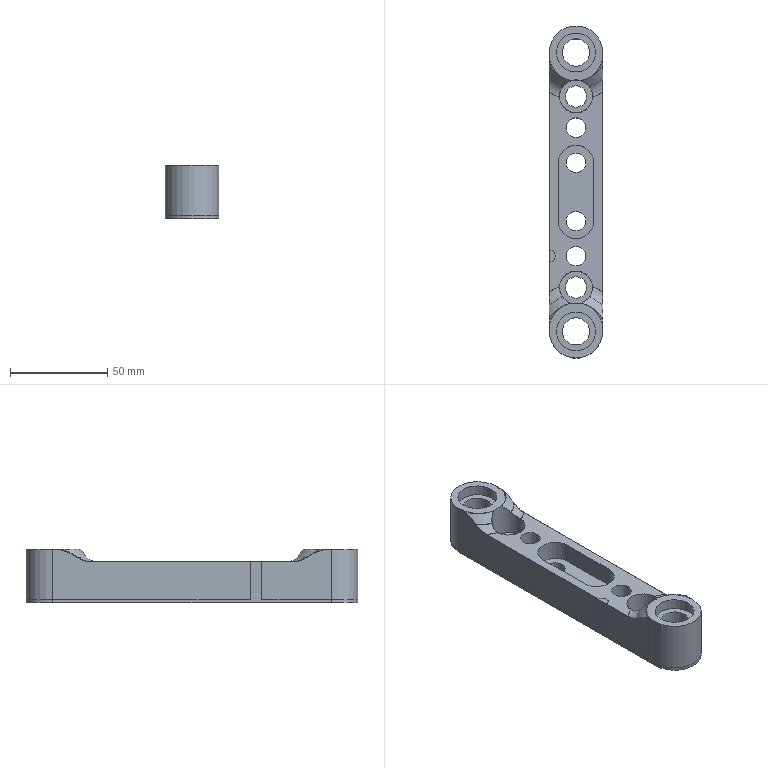NC program | NX | posted with a generic post | part box 27.4 x 170.48 x 27.5 mm
Lines 5462 to 6209 of 10888:
(ADAPTIVE_MILLING_COPY , TOOL : D8开粗)
N10886 T06 M6
N10888 G54
N10890 G17 G0 G90 X-73.84 Y2.769 B0. C0. S4000 M3
N10892 G43 Z30. H6
N10894 Z3.
N10896 G94 G3 X-73.84 Y2.769 Z2.605 I2.3 J-2.77 F1500.
N10898 X-73.84 Y2.769 Z2.21 I2.3 J-2.77
N10900 X-73.84 Y2.769 Z1.816 I2.3 J-2.77
N10902 X-73.84 Y2.769 Z1.421 I2.3 J-2.77
N10904 X-73.84 Y2.769 Z1.026 I2.3 J-2.77
N10906 X-73.84 Y2.769 Z0.631 I2.3 J-2.77
N10908 X-73.84 Y2.769 Z0.236 I2.3 J-2.77
N10910 X-73.84 Y2.769 Z-0.159 I2.3 J-2.77
N10912 X-73.84 Y2.769 Z-0.553 I2.3 J-2.77
N10914 X-73.84 Y2.769 Z-0.948 I2.3 J-2.77
N10916 X-73.84 Y2.769 Z-1.343 I2.3 J-2.77
N10918 X-73.84 Y2.769 Z-1.738 I2.3 J-2.77
N10920 X-73.84 Y2.769 Z-2.133 I2.3 J-2.77
N10922 X-73.84 Y2.769 Z-2.528 I2.3 J-2.77
N10924 X-73.84 Y2.769 Z-2.922 I2.3 J-2.77
N10926 X-73.84 Y2.769 Z-3.317 I2.3 J-2.77
N10928 X-73.84 Y2.769 Z-3.712 I2.3 J-2.77
N10930 X-73.84 Y2.769 Z-4.107 I2.3 J-2.77
N10932 X-73.84 Y2.769 Z-4.502 I2.3 J-2.77
N10934 X-71.541 Y3.599 Z-4.853 R-3.6
N10936 X-68.26 Y-1.603 R-3.625
N10938 X-74.92 Y-1.63 R-3.701
N10940 X-70.356 Y3.616 R-3.777
N10942 X-74.119 Y-2.909 R3.84
N10944 X-70.299 Y3.738 R-3.912
N10946 X-74.023 Y-3.163 R3.976
N10948 X-70.052 Y3.789 R-4.045
N10950 X-73.899 Y-3.423 R4.111
N10952 X-70.025 Y3.926 R-4.182
N10954 X-73.744 Y-3.685 R4.249
N10956 X-70.014 Y4.072 R-4.321
N10958 X-73.558 Y-3.949 R4.39
N10960 X-69.804 Y4.14 R-4.462
N10962 X-75.75 Y1.741 R4.533
N10964 X-73.34 Y-4.208 R4.533
N10966 X-69.824 Y4.306 R-4.606
N10968 X-72.864 Y-4.535 R-4.681
N10970 X-70.316 Y4.629 R-4.756
N10972 X-72.337 Y-4.809 R-4.832
N10974 X-71.101 Y4.925 R-4.909
N10976 X-71.272 Y-5.021 R-4.987
N10978 X-72.435 Y5.03 R-5.067
N10980 X-69.696 Y-4.845 R-5.148
N10982 X-74.43 Y4.417 R-5.229
N10984 X-67.181 Y-3.098 R-5.315
N10986 X-77.004 Y-0.069 R-5.404
N10988 X-66.868 Y2.951 R-5.495
N10990 X-75.057 Y-4.408 R-5.584
N10992 X-65.915 Y-0.707 R5.654
N10994 X-74.818 Y4.656 R5.678
N10996 X-76.45 Y2.889 R6.452
N10998 X-66.026 Y-1.422 R-5.695
N11000 X-65.913 Y0.863 R6.414
N11002 X-66.959 Y3.373 R6.034
N11004 X-69.395 Y5.276 R5.646
N11006 X-70.5 Y4.622 R0.808
N11008 G1 X-70.622 Y3.585
N11010 X-70.64 Y3.436 Z-4.849
N11012 X-70.657 Y3.287 Z-4.838
N11014 X-70.675 Y3.138 Z-4.819
N11016 X-70.693 Y2.989 Z-4.792
N11018 X-70.71 Y2.84 Z-4.758
N11020 X-70.728 Y2.691 Z-4.715
N11022 X-70.745 Y2.542 Z-4.663
N11024 X-70.763 Y2.393 Z-4.602
N11026 X-70.781 Y2.245 Z-4.532
N11028 X-70.798 Y2.096 Z-4.451
N11030 X-70.816 Y1.947 Z-4.358
N11032 X-70.833 Y1.798 Z-4.253
N11034 X-70.851 Y1.649 Z-4.133
N11036 X-70.869 Y1.5 Z-3.995
N11038 X-70.886 Y1.351 Z-3.837
N11040 X-70.904 Y1.202 Z-3.653
N11042 X-70.921 Y1.053 Z-3.433
N11044 X-70.939 Y0.904 Z-3.161
N11046 X-70.956 Y0.755 Z-2.79
N11048 X-70.974 Y0.606 Z-1.853
N11050 G0 Z30.
N11052 X69.239 Y2.771
N11054 Z3.
N11056 G3 X69.239 Y2.771 Z2.605 I2.3 J-2.77
N11058 X69.239 Y2.771 Z2.21 I2.3 J-2.77
N11060 X69.239 Y2.771 Z1.816 I2.3 J-2.77
N11062 X69.239 Y2.771 Z1.421 I2.3 J-2.77
N11064 X69.239 Y2.771 Z1.026 I2.3 J-2.77
N11066 X69.239 Y2.771 Z0.631 I2.3 J-2.77
N11068 X69.239 Y2.771 Z0.236 I2.3 J-2.77
N11070 X69.239 Y2.771 Z-0.159 I2.3 J-2.77
N11072 X69.239 Y2.771 Z-0.553 I2.3 J-2.77
N11074 X69.239 Y2.771 Z-0.948 I2.3 J-2.77
N11076 X69.239 Y2.771 Z-1.343 I2.3 J-2.77
N11078 X69.239 Y2.771 Z-1.738 I2.3 J-2.77
N11080 X69.239 Y2.771 Z-2.133 I2.3 J-2.77
N11082 X69.239 Y2.771 Z-2.528 I2.3 J-2.77
N11084 X69.239 Y2.771 Z-2.922 I2.3 J-2.77
N11086 X69.239 Y2.771 Z-3.317 I2.3 J-2.77
N11088 X69.239 Y2.771 Z-3.712 I2.3 J-2.77
N11090 X69.239 Y2.771 Z-4.107 I2.3 J-2.77
N11092 X69.239 Y2.771 Z-4.502 I2.3 J-2.77
N11094 X71.539 Y3.601 Z-4.853 R-3.6
N11096 X74.82 Y-1.601 R-3.625
N11098 X68.16 Y-1.627 R-3.701
N11100 X72.723 Y3.617 R-3.777
N11102 X68.803 Y-2.759 R3.839
N11104 X72.572 Y3.806 R-3.912
N11106 X69.234 Y-3.292 R3.977
N11108 X72.819 Y3.87 R-4.046
N11110 X69.182 Y-3.422 R4.112
N11112 X73.053 Y3.929 R-4.182
N11114 X69.146 Y-3.563 R4.249
N11116 X73.064 Y4.075 R-4.32
N11118 X69.123 Y-3.716 R4.389
N11120 X73.275 Y4.142 R-4.461
N11122 X69.525 Y-4.11 R4.533
N11124 X73.036 Y4.39 R-4.607
N11126 X69.764 Y-4.376 R4.68
N11128 X72.766 Y4.628 R-4.755
N11130 X66.845 Y1.221 R4.831
N11132 X70.267 Y-4.704 R4.831
N11134 X72.224 Y4.895 R-4.907
N11136 X71.312 Y-5.02 R-4.985
N11138 X71.388 Y5.1 R-5.063
N11140 X72.905 Y-4.998 R-5.144
N11142 X69.316 Y4.783 R-5.226
N11144 X75.409 Y-3.684 R-5.31
N11146 X66.354 Y1.7 R-5.398
N11148 X76.959 Y1.04 R-5.488
N11150 X67.106 Y-3.479 R-5.578
N11152 X77.164 Y-0.712 R5.653
N11154 X71.272 Y5.688 R5.681
N11156 X66.021 Y1.396 R5.729
N11158 X67.16 Y-3.638 R5.816
N11160 X74.269 Y-4.999 R5.748
N11162 X76.644 Y-2.519 R6.075
N11164 X77.231 Y-0.106 R6.229
N11166 X77.084 Y1.308 R7.829
N11168 X73.315 Y5.41 R5.784
N11170 X72.26 Y4.682 R0.808
N11172 G1 X72.207 Y3.631
N11174 X72.199 Y3.481 Z-4.849
N11176 X72.191 Y3.332 Z-4.838
N11178 X72.184 Y3.182 Z-4.819
N11180 X72.176 Y3.032 Z-4.792
N11182 X72.169 Y2.882 Z-4.758
N11184 X72.161 Y2.732 Z-4.715
N11186 X72.153 Y2.583 Z-4.663
N11188 X72.146 Y2.433 Z-4.602
N11190 X72.138 Y2.283 Z-4.532
N11192 X72.13 Y2.133 Z-4.451
N11194 X72.123 Y1.983 Z-4.358
N11196 X72.115 Y1.833 Z-4.253
N11198 X72.108 Y1.684 Z-4.133
N11200 X72.1 Y1.534 Z-3.995
N11202 X72.092 Y1.384 Z-3.837
N11204 X72.085 Y1.234 Z-3.653
N11206 X72.077 Y1.084 Z-3.433
N11208 X72.069 Y0.935 Z-3.161
N11210 X72.062 Y0.785 Z-2.79
N11212 X72.054 Y0.635 Z-1.853
N11214 G0 Z30.
N11216 X-46.689 Y-2.761
N11218 Z3.
N11220 G3 X-46.689 Y-2.761 Z2.605 I-2.311 J2.76
N11222 X-46.689 Y-2.761 Z2.21 I-2.311 J2.76
N11224 X-46.689 Y-2.761 Z1.816 I-2.311 J2.76
N11226 X-46.689 Y-2.761 Z1.421 I-2.311 J2.76
N11228 X-46.689 Y-2.761 Z1.026 I-2.311 J2.76
N11230 X-46.689 Y-2.761 Z0.631 I-2.311 J2.76
N11232 X-46.689 Y-2.761 Z0.236 I-2.311 J2.76
N11234 X-46.689 Y-2.761 Z-0.159 I-2.311 J2.76
N11236 X-46.689 Y-2.761 Z-0.553 I-2.311 J2.76
N11238 X-46.689 Y-2.761 Z-0.948 I-2.311 J2.76
N11240 X-46.689 Y-2.761 Z-1.343 I-2.311 J2.76
N11242 X-46.689 Y-2.761 Z-1.738 I-2.311 J2.76
N11244 X-46.689 Y-2.761 Z-2.133 I-2.311 J2.76
N11246 X-46.689 Y-2.761 Z-2.528 I-2.311 J2.76
N11248 X-46.689 Y-2.761 Z-2.922 I-2.311 J2.76
N11250 X-46.689 Y-2.761 Z-3.317 I-2.311 J2.76
N11252 X-46.689 Y-2.761 Z-3.712 I-2.311 J2.76
N11254 X-46.689 Y-2.761 Z-4.107 I-2.311 J2.76
N11256 X-46.689 Y-2.761 Z-4.502 I-2.311 J2.76
N11258 X-46.689 Y-2.761 Z-4.896 I-2.311 J2.76
N11260 X-46.689 Y-2.761 Z-5.291 I-2.311 J2.76
N11262 X-46.689 Y-2.761 Z-5.686 I-2.311 J2.76
N11264 X-46.689 Y-2.761 Z-6.081 I-2.311 J2.76
N11266 X-46.689 Y-2.761 Z-6.476 I-2.311 J2.76
N11268 X-46.689 Y-2.761 Z-6.871 I-2.311 J2.76
N11270 X-46.689 Y-2.761 Z-7.265 I-2.311 J2.76
N11272 X-46.689 Y-2.761 Z-7.66 I-2.311 J2.76
N11274 X-46.689 Y-2.761 Z-8.055 I-2.311 J2.76
N11276 X-46.689 Y-2.761 Z-8.45 I-2.311 J2.76
N11278 X-46.689 Y-2.761 Z-8.845 I-2.311 J2.76
N11280 X-46.689 Y-2.761 Z-9.24 I-2.311 J2.76
N11282 X-46.689 Y-2.761 Z-9.634 I-2.311 J2.76
N11284 X-46.689 Y-2.761 Z-10.029 I-2.311 J2.76
N11286 X-46.689 Y-2.761 Z-10.424 I-2.311 J2.76
N11288 X-46.689 Y-2.761 Z-10.819 I-2.311 J2.76
N11290 X-46.689 Y-2.761 Z-11.214 I-2.311 J2.76
N11292 X-46.689 Y-2.761 Z-11.608 I-2.311 J2.76
N11294 X-46.689 Y-2.761 Z-12.003 I-2.311 J2.76
N11296 X-46.689 Y-2.761 Z-12.398 I-2.311 J2.76
N11298 X-46.689 Y-2.761 Z-12.793 I-2.311 J2.76
N11300 X-46.689 Y-2.761 Z-13.188 I-2.311 J2.76
N11302 X-46.689 Y-2.761 Z-13.583 I-2.311 J2.76
N11304 X-46.689 Y-2.761 Z-13.977 I-2.311 J2.76
N11306 X-46.689 Y-2.761 Z-14.372 I-2.311 J2.76
N11308 X-46.689 Y-2.761 Z-14.767 I-2.311 J2.76
N11310 X-46.689 Y-2.761 Z-15.162 I-2.311 J2.76
N11312 X-46.689 Y-2.761 Z-15.557 I-2.311 J2.76
N11314 X-46.689 Y-2.761 Z-15.952 I-2.311 J2.76
N11316 X-46.689 Y-2.761 Z-16.346 I-2.311 J2.76
N11318 X-49. Y3.6 Z-16.5 R3.6
N11320 X-45.719 Y-1.602 R-3.625
N11322 X-52.283 Y-1.818 R-3.701
N11324 X-47.816 Y3.616 R-3.778
N11326 X-51.736 Y-2.76 R3.838
N11328 X-47.76 Y3.738 R-3.911
N11330 X-51.65 Y-3.021 R3.972
N11332 X-47.514 Y3.789 R-4.044
N11334 X-51.709 Y-3.149 R4.107
N11336 X-48.604 Y-4.149 R4.159
N11338 X-50.93 Y3.721 R-4.18
N11340 X-53.159 Y-0.53 R4.22
N11342 X-52.029 Y-2.882 R4.227
N11344 X-50.296 Y-3.988 R3.884
N11346 X-47.443 Y-3.89 R4.401
N11348 X-44.825 Y-0.368 R4.251
N11350 X-47.407 Y3.877 R4.225
N11352 X-48.508 Y3.221 R0.808
N11354 G1 X-48.634 Y2.16
N11356 X-48.652 Y2.011 Z-16.496
N11358 X-48.67 Y1.862 Z-16.485
N11360 X-48.687 Y1.713 Z-16.466
N11362 X-48.705 Y1.564 Z-16.439
N11364 X-48.723 Y1.415 Z-16.405
N11366 X-48.74 Y1.266 Z-16.362
N11368 X-48.758 Y1.117 Z-16.31
N11370 X-48.776 Y0.968 Z-16.25
N11372 X-48.794 Y0.819 Z-16.179
N11374 X-48.811 Y0.67 Z-16.098
N11376 X-48.829 Y0.521 Z-16.005
N11378 X-48.847 Y0.372 Z-15.9
N11380 X-48.864 Y0.223 Z-15.78
N11382 X-48.882 Y0.074 Z-15.642
N11384 X-48.9 Y-0.075 Z-15.484
N11386 X-48.917 Y-0.224 Z-15.3
N11388 X-48.935 Y-0.373 Z-15.08
N11390 X-48.953 Y-0.522 Z-14.808
N11392 X-48.97 Y-0.67 Z-14.437
N11394 X-48.988 Y-0.819 Z-13.5
N11396 G0 Z30.
N11398 X-48.921 Y0.758
N11400 Z-2.824
N11402 G1 X-48.949 Y0.611 Z-3.76
N11404 X-48.978 Y0.463 Z-4.131
N11406 X-49.006 Y0.316 Z-4.404
N11408 X-49.035 Y0.169 Z-4.624
N11410 X-49.063 Y0.021 Z-4.808
N11412 X-49.091 Y-0.126 Z-4.966
N11414 X-49.12 Y-0.273 Z-5.103
N11416 X-49.148 Y-0.421 Z-5.224
N11418 X-49.176 Y-0.568 Z-5.329
N11420 X-49.205 Y-0.715 Z-5.422
N11422 X-49.233 Y-0.862 Z-5.503
N11424 X-49.261 Y-1.01 Z-5.573
N11426 X-49.29 Y-1.157 Z-5.634
N11428 X-49.318 Y-1.304 Z-5.685
N11430 X-49.347 Y-1.452 Z-5.728
N11432 X-49.375 Y-1.599 Z-5.763
N11434 X-49.403 Y-1.746 Z-5.79
N11436 X-49.432 Y-1.893 Z-5.808
N11438 X-49.46 Y-2.041 Z-5.82
N11440 X-49.488 Y-2.188 Z-5.824
N11442 X-49.758 Y-3.586
N11444 G3 X-49.407 Y-4.414 R0.809
N11446 G2 X-47.983 Y-5.539 R6.465
N11448 X-47.123 Y-7.109 R4.659
N11450 X-47.037 Y-8.898 R4.659
N11452 X-48.987 Y-13.563 R17.207
N11454 X-50.821 Y-15.909 R7.143
N11456 X-51.757 Y-16.934 R6.606
N11458 G1 X-52.621 Y-17.475
N11460 G2 X-53.772 Y-17.834 R7.888
N11462 G3 X-54.224 Y-19.168 R0.8
N11464 X-53.705 Y-19.423 Z-5.786 R0.859
N11466 G1 X-52.722 Y-19.601 Z-5.724
N11468 X-51.383 Y-19.843 F15000.
N11470 G3 X-50.675 Y-19.622 R0.802
N11472 G1 X-49.772 Y-18.721
N11474 X-48.88 Y-17.81
N11476 G3 X-46.917 Y-15.066 R13.735
N11478 G1 X-45.249 Y-11.995
N11480 G3 X-45.158 Y-11.511 R0.81
N11482 G1 X-45.332 Y-10.155
N11484 X-45.488 Y-8.97 Z-5.799 F1500.
N11486 G3 X-45.654 Y-8.617 Z-5.824 R0.815
N11488 X-47.037 Y-8.898 R0.8
N11490 G1 X-47.296 Y-9.762
N11492 X-48.34 Y-12.034
N11494 X-49.59 Y-14.187
N11496 X-50.856 Y-15.955
N11498 G3 X-50.824 Y-16.938 R0.808
N11500 G1 X-49.981 Y-17.965
N11502 X-49.886 Y-18.081 Z-5.82
N11504 X-49.79 Y-18.197 Z-5.808
N11506 X-49.695 Y-18.313 Z-5.79
N11508 X-49.6 Y-18.429 Z-5.763
N11510 X-49.505 Y-18.545 Z-5.728
N11512 X-49.41 Y-18.661 Z-5.685
N11514 X-49.314 Y-18.777 Z-5.634
N11516 X-49.219 Y-18.892 Z-5.573
N11518 X-49.124 Y-19.008 Z-5.503
N11520 X-49.029 Y-19.124 Z-5.422
N11522 X-48.934 Y-19.24 Z-5.329
N11524 X-48.839 Y-19.356 Z-5.224
N11526 X-48.743 Y-19.472 Z-5.103
N11528 X-48.648 Y-19.588 Z-4.966
N11530 X-48.553 Y-19.704 Z-4.808
N11532 X-48.458 Y-19.82 Z-4.624
N11534 X-48.363 Y-19.936 Z-4.404
N11536 X-48.267 Y-20.052 Z-4.131
N11538 X-48.172 Y-20.168 Z-3.76
N11540 X-48.077 Y-20.284 Z-2.824
N11542 G0 Z30.
N11544 X-47.959 Y0.175
N11546 Z-1.853
N11548 G1 X-48.068 Y0.071 Z-2.79
N11550 X-48.176 Y-0.033 Z-3.161
N11552 X-48.284 Y-0.137 Z-3.433
N11554 X-48.392 Y-0.241 Z-3.653
N11556 X-48.501 Y-0.345 Z-3.837
N11558 X-48.609 Y-0.448 Z-3.995
N11560 X-48.717 Y-0.552 Z-4.133
N11562 X-48.825 Y-0.656 Z-4.253
N11564 X-48.934 Y-0.76 Z-4.358
N11566 X-49.042 Y-0.864 Z-4.451
N11568 X-49.15 Y-0.968 Z-4.532
N11570 X-49.258 Y-1.071 Z-4.602
N11572 X-49.367 Y-1.175 Z-4.663
N11574 X-49.475 Y-1.279 Z-4.715
N11576 X-49.583 Y-1.383 Z-4.758
N11578 X-49.691 Y-1.487 Z-4.792
N11580 X-49.799 Y-1.591 Z-4.819
N11582 X-49.908 Y-1.695 Z-4.838
N11584 X-50.016 Y-1.798 Z-4.849
N11586 X-50.124 Y-1.902 Z-4.853
N11588 X-50.877 Y-2.624
N11590 G3 X-50.788 Y-3.864 R0.808
N11592 G2 X-49.389 Y-4.957 R7.32
N11594 X-48.139 Y-8.974 R5.437
N11596 X-49.59 Y-13.357 R10.542
N11598 X-51.081 Y-15.5 R9.698
N11600 X-54.173 Y-17.113 R5.957
N11602 G1 X-54.468 Y-17.163
N11604 G3 X-54.874 Y-18.349 R0.8
N11606 X-54.229 Y-18.72 Z-4.804 R0.831
N11608 G1 X-53.419 Y-18.824 Z-4.753
N11610 X-51.831 Y-19.029 F15000.
N11612 G3 X-51.371 Y-18.951 R0.813
N11614 G1 X-51.039 Y-18.785
N11616 X-50.712 Y-18.609
N11618 G3 X-50.146 Y-18.141 R2.814
N11620 G1 X-49.146 Y-17.04
N11622 G3 X-47.722 Y-15.022 R13.499
N11624 G1 X-46.991 Y-13.731
N11626 G3 X-45.702 Y-9.541 R12.053
N11628 G1 X-45.636 Y-8.975
N11630 X-45.58 Y-8.407
N11632 G3 X-46.22 Y-5.513 R5.51
N11634 G1 X-47.029 Y-3.995
N11636 G3 X-47.42 Y-3.636 R0.807
N11638 G1 X-48.61 Y-3.128
N11640 X-49.247 Y-2.853 Z-4.797 F1500.
N11642 X-49.889 Y-2.588 Z-4.84
N11644 X-49.986 Y-2.563 Z-4.847
N11646 X-50.085 Y-2.547 Z-4.853
N11648 G3 X-50.605 Y-3.995 R0.8
N11650 G2 X-49.406 Y-5.36 R4.728
N11652 G1 X-49.281 Y-5.504
N11654 G2 X-48.811 Y-6.618 R5.434
N11656 X-49.444 Y-12.028 R9.131
N11658 X-51.782 Y-15.275 R7.349
N11660 X-52.871 Y-15.927 R4.
N11662 G1 X-53.231 Y-16.028
N11664 G3 X-53.433 Y-17.303 R0.8
N11666 X-52.692 Y-17.525 Z-4.802 R0.832
N11668 G1 X-51.914 Y-17.431 Z-4.753
N11670 X-50.841 Y-17.302 F15000.
N11672 G3 X-50.208 Y-16.838 R0.801
N11674 G1 X-46.169 Y-7.93
N11676 G3 X-46.292 Y-7.077 R0.801
N11678 G1 X-46.826 Y-6.458
N11680 X-47.192 Y-6.027 Z-4.789 F1500.
N11682 X-47.569 Y-5.607 Z-4.824
N11684 G3 X-47.982 Y-5.419 Z-4.853 R0.833
N11686 X-48.879 Y-6.365 R0.8
N11688 G1 X-48.696 Y-7.298
N11690 G2 X-49.35 Y-10.718 R9.889
N11692 X-51.161 Y-13.887 R7.958
N11694 X-51.926 Y-14.418 R1.888
N11696 G3 X-51.719 Y-15.869 R0.8
N11698 X-51.087 Y-15.785 Z-4.812 R0.847
N11700 G1 X-50.244 Y-15.379 Z-4.753
N11702 X-48.569 Y-14.573 F15000.
N11704 X-48.454 Y-14.504
N11706 X-48.35 Y-14.418
N11708 X-48.105 Y-14.174
N11710 X-47.868 Y-13.923
N11712 G3 X-47.508 Y-13.239 R1.968
N11714 G1 X-46.953 Y-11.344
N11716 X-46.927 Y-11.195
N11718 X-46.925 Y-11.043
N11720 X-47.064 Y-9.597
N11722 X-47.19 Y-8.336 Z-4.833 F1500.
N11724 X-47.233 Y-8.182 Z-4.843
N11726 X-47.306 Y-8.038 Z-4.853
N11728 G3 X-48.741 Y-8.247 R0.8
N11730 G1 X-49.014 Y-9.158
N11732 X-49.029 Y-9.192
N11734 X-49.059 Y-9.261
N11736 G3 X-47.42 Y-9.905 R-0.881
N11738 X-49.045 Y-9.226 R-0.88
N11740 X-48.04 Y-10.396 R0.83
N11742 X-47.605 Y-9.117 R0.875
N11744 X-49.075 Y-9.295 R0.83
N11746 G1 X-49.093 Y-9.428
N11748 X-49.092 Y-9.562
N11750 X-48.919 Y-11.196
N11752 X-48.805 Y-12.219 Z-4.788
N11754 G3 X-48.528 Y-12.692 Z-4.753 R0.802
N11756 X-47.272 Y-12.357 R0.801 F15000.
N11758 X-47.213 Y-11.933 R0.818
N11760 G1 X-47.411 Y-10.45
N11762 X-47.553 Y-9.427 Z-4.818 F1500.
N11764 G3 X-47.839 Y-8.964 Z-4.853 R0.802
N11766 X-49.06 Y-9.26 R0.8
N11768 G1 X-49.147 Y-9.546
N11770 G3 X-48.83 Y-8.989 R-0.797
N11772 X-49.076 Y-9.294 R0.831
N11774 X-49.374 Y-10.258 R3.935
N11776 G2 X-50.275 Y-12.355 R10.996
N11778 G3 X-50.319 Y-13.032 R0.802
N11780 X-49.325 Y-13.505 Z-4.777 R0.814
N11782 G1 X-48.955 Y-13.422 Z-4.753
N11784 X-47.319 Y-13.055 F15000.
N11786 G3 X-46.699 Y-12.355 R0.801
N11788 G1 X-46.674 Y-12.118
N11790 X-46.68 Y-11.879
N11792 X-46.708 Y-11.774
N11794 X-46.746 Y-11.672
N11796 X-47.367 Y-10.365
N11798 X-47.581 Y-9.907 Z-4.785 F1500.
N11800 X-47.808 Y-9.456 Z-4.817
N11802 G3 X-48.269 Y-9.127 Z-4.853 R0.821
N11804 X-49.201 Y-9.567 R0.8
N11806 G2 X-51.416 Y-13.638 R27.243
N11808 X-53.898 Y-16.683 R26.39
N11810 X-55.596 Y-17.679 R4.037
N11812 G3 X-56.556 Y-17.915 R8.77
N11814 X-57.269 Y-18.893 R0.808
N11816 G1 X-57.036 Y-19.956
N11818 X-57.003 Y-20.103 Z-4.849
N11820 X-56.971 Y-20.249 Z-4.838
N11822 X-56.939 Y-20.396 Z-4.819
N11824 X-56.907 Y-20.542 Z-4.792
N11826 X-56.875 Y-20.689 Z-4.758
N11828 X-56.843 Y-20.835 Z-4.715
N11830 X-56.81 Y-20.982 Z-4.663
N11832 X-56.778 Y-21.128 Z-4.602
N11834 X-56.746 Y-21.275 Z-4.532
N11836 X-56.714 Y-21.422 Z-4.451
N11838 X-56.682 Y-21.568 Z-4.358
N11840 X-56.65 Y-21.715 Z-4.253
N11842 X-56.617 Y-21.861 Z-4.133
N11844 X-56.585 Y-22.008 Z-3.995
N11846 X-56.553 Y-22.154 Z-3.837
N11848 X-56.521 Y-22.301 Z-3.653
N11850 X-56.489 Y-22.447 Z-3.433
N11852 X-56.456 Y-22.594 Z-3.161
N11854 X-56.424 Y-22.74 Z-2.79
N11856 X-56.392 Y-22.887 Z-1.853
N11858 G0 Z30.
N11860 X-54.862 Y22.912
N11862 Z-2.824
N11864 G1 X-54.844 Y22.763 Z-3.76
N11866 X-54.825 Y22.614 Z-4.131
N11868 X-54.807 Y22.465 Z-4.404
N11870 X-54.788 Y22.316 Z-4.624
N11872 X-54.77 Y22.168 Z-4.808
N11874 X-54.751 Y22.019 Z-4.966
N11876 X-54.732 Y21.87 Z-5.103
N11878 X-54.714 Y21.721 Z-5.224
N11880 X-54.695 Y21.572 Z-5.329
N11882 X-54.677 Y21.423 Z-5.422
N11884 X-54.658 Y21.274 Z-5.503
N11886 X-54.64 Y21.126 Z-5.573
N11888 X-54.621 Y20.977 Z-5.634
N11890 X-54.603 Y20.828 Z-5.685
N11892 X-54.584 Y20.679 Z-5.728
N11894 X-54.566 Y20.53 Z-5.763
N11896 X-54.547 Y20.381 Z-5.79
N11898 X-54.529 Y20.232 Z-5.808
N11900 X-54.51 Y20.084 Z-5.82
N11902 X-54.492 Y19.935 Z-5.824
N11904 X-54.312 Y18.492
N11906 G3 X-53.672 Y17.8 R0.809
N11908 G2 X-50.954 Y16.146 R4.679
N11910 X-47.602 Y10.813 R19.232
N11912 G1 X-47.403 Y9.993
N11914 G2 X-47.041 Y8.831 R6.197
N11916 G1 X-47.006 Y7.872
N11918 X-47.193 Y6.93
N11920 X-47.59 Y6.056
N11922 X-48.176 Y5.296
N11924 G2 X-49.282 Y4.487 R5.681
N11926 G3 X-48.575 Y3.055 R0.8
N11928 G1 X-48.385 Y3.136
N11930 X-46.923 Y3.761 Z-5.724
N11932 X-46.462 Y3.954 F15000.
N11934 X-46.007 Y4.161
N11936 G3 X-45.706 Y4.487 R0.816
N11938 G1 X-45.092 Y5.734
N11940 G3 X-44.505 Y7.495 R8.63
N11942 X-44.596 Y9.138 R3.556
N11944 G1 X-45.071 Y10.744
N11946 X-45.56 Y12.346
N11948 G3 X-47.042 Y15.307 R12.243
N11950 G1 X-48.121 Y16.886
N11952 G3 X-48.465 Y17.169 R0.816
N11954 G1 X-49.705 Y17.704
N11956 X-50.87 Y18.201 Z-5.803 F1500.
N11958 X-51.027 Y18.238 Z-5.813
N11960 X-51.187 Y18.244 Z-5.824
N11962 G3 X-51.697 Y16.886 R0.8
N11964 G1 X-51.056 Y16.231
N11966 X-49.597 Y14.197
N11968 X-48.339 Y12.032
N11970 X-47.4 Y9.987
N11972 G3 X-46.576 Y9.521 R0.809
N11974 G1 X-45.211 Y9.673
N11976 X-45.062 Y9.69 Z-5.82
N11978 X-44.913 Y9.706 Z-5.808
N11980 X-44.764 Y9.723 Z-5.79
N11982 X-44.615 Y9.739 Z-5.763
N11984 X-44.466 Y9.756 Z-5.728
N11986 X-44.317 Y9.772 Z-5.685
N11988 X-44.168 Y9.789 Z-5.634
N11990 X-44.019 Y9.806 Z-5.573
N11992 X-43.87 Y9.822 Z-5.503
N11994 X-43.721 Y9.839 Z-5.422
N11996 X-43.572 Y9.855 Z-5.329
N11998 X-43.422 Y9.872 Z-5.224
N12000 X-43.273 Y9.888 Z-5.103
N12002 X-43.124 Y9.905 Z-4.966
N12004 X-42.975 Y9.922 Z-4.808
N12006 X-42.826 Y9.938 Z-4.624
N12008 X-42.677 Y9.955 Z-4.404
N12010 X-42.528 Y9.971 Z-4.131
N12012 X-42.379 Y9.988 Z-3.76
N12014 X-42.23 Y10.004 Z-2.824
N12016 G0 Z30.
N12018 X-58.118 Y22.882
N12020 Z-1.853
N12022 G1 X-58.083 Y22.737 Z-2.79
N12024 X-58.048 Y22.591 Z-3.161
N12026 X-58.013 Y22.445 Z-3.433
N12028 X-57.978 Y22.299 Z-3.653
N12030 X-57.943 Y22.153 Z-3.837
N12032 X-57.908 Y22.007 Z-3.995
N12034 X-57.873 Y21.861 Z-4.133
N12036 X-57.838 Y21.715 Z-4.253
N12038 X-57.803 Y21.569 Z-4.358
N12040 X-57.768 Y21.424 Z-4.451
N12042 X-57.734 Y21.278 Z-4.532
N12044 X-57.699 Y21.132 Z-4.602
N12046 X-57.664 Y20.986 Z-4.663
N12048 X-57.629 Y20.84 Z-4.715
N12050 X-57.594 Y20.694 Z-4.758
N12052 X-57.559 Y20.548 Z-4.792
N12054 X-57.524 Y20.402 Z-4.819
N12056 X-57.489 Y20.257 Z-4.838
N12058 X-57.454 Y20.111 Z-4.849
N12060 X-57.419 Y19.965 Z-4.853
N12062 X-57.067 Y18.496
N12064 G3 X-56.491 Y17.903 R0.809
N12066 G2 X-54.675 Y17.6 R85.338
N12068 X-51.159 Y15.394 R7.558
N12070 X-48.095 Y10.587 R16.006
N12072 X-48.861 Y6.508 R4.534
N12074 G1 X-48.892 Y6.44
N12076 G3 X-48.398 Y5.413 R0.8
N12078 X-47.651 Y5.532 Z-4.804 R0.829
N12080 G1 X-46.971 Y5.96 Z-4.753
N12082 X-45.812 Y6.688 F15000.
N12084 G3 X-45.438 Y7.366 R0.801
N12086 G1 X-45.435 Y8.523
N12088 X-45.446 Y9.681
N12090 G3 X-46.019 Y12.032 R6.831
N12092 X-46.827 Y13.502 R10.603
N12094 X-49.226 Y16.737 R25.639
N12096 X-51.752 Y18.967 R13.636
N12098 G1 X-53.854 Y20.403
N12100 G3 X-54.709 Y20.433 R0.801
N12102 G1 X-55.803 Y19.792
N12104 X-56.222 Y19.549 Z-4.783 F1500.
N12106 X-56.635 Y19.297 Z-4.814
N12108 G3 X-56.962 Y18.79 Z-4.853 R0.8
N12110 X-56.382 Y17.874 R0.8
N12112 G2 X-55.111 Y17.526 R12.291
N12114 X-50. Y13.253 R11.538
N12116 X-48.836 Y10.632 R5.92
N12118 X-48.869 Y8.807 R4.816
N12120 G3 X-47.868 Y8.021 R0.8
N12122 X-47.305 Y8.545 Z-4.803 R0.833
N12124 G1 X-46.986 Y9.267 Z-4.753
N12126 X-46.566 Y10.218 F15000.
N12128 G3 X-46.657 Y11.019 R0.801
N12130 G1 X-52.755 Y19.212
N12132 G3 X-53.566 Y19.516 R0.801
N12134 G1 X-54.378 Y19.34
N12136 X-55.342 Y19.127 Z-4.815 F1500.
N12138 G3 X-55.803 Y18.763 Z-4.853 R0.801
N12140 X-55.465 Y17.647 R0.8
N12142 G2 X-54.148 Y16.912 R7.674
N12144 X-51.429 Y14.452 R13.317
N12146 X-49.62 Y11.122 R7.15
N12148 G1 X-49.637 Y10.636
N12150 G3 X-48.376 Y10.058 R0.8
N12152 X-48.037 Y10.68 Z-4.807 R0.841
N12154 G1 X-47.923 Y11.53 Z-4.753
N12156 X-47.703 Y13.155 F15000.
N12158 G3 X-47.849 Y13.733 R0.805
N12160 G1 X-50.95 Y17.993
N12162 G3 X-51.539 Y18.32 R0.803
N12164 G1 X-52.898 Y18.42
N12166 X-53.909 Y18.489 Z-4.817 F1500.
N12168 G3 X-54.435 Y18.289 Z-4.853 R0.801
N12170 X-54.405 Y17.068 R0.8
N12172 G1 X-53.81 Y16.59
N12174 G3 X-52.159 Y14.928 R15.088
N12176 G2 X-50.604 Y12.914 R11.851
N12178 G3 X-49.909 Y12.501 R0.882
N12180 X-48.991 Y13.534 Z-4.753 R0.882
N12182 X-49.186 Y13.949 R0.899 F15000.
N12184 G1 X-49.55 Y14.377
N12186 X-50.578 Y15.589 Z-4.853 F1500.
N12188 X-51.459 Y16.627
N12190 G3 X-52.831 Y15.526 R0.88
N12192 G2 X-48.997 Y9.087 R25.776
N12194 X-49.287 Y5.489 R4.167
N12196 G3 X-49.821 Y4.728 R6.444
N12198 G2 X-50.811 Y3.844 R5.841
N12200 G3 X-51.053 Y2.803 R0.808
N12202 G1 X-50.439 Y1.664
N12204 X-50.368 Y1.532 Z-4.849
N12206 X-50.296 Y1.4 Z-4.838
N12208 X-50.225 Y1.268 Z-4.819
N12210 X-50.154 Y1.136 Z-4.792
N12212 X-50.083 Y1.004 Z-4.758
N12214 X-50.011 Y0.872 Z-4.715
N12216 X-49.94 Y0.74 Z-4.663
N12218 X-49.869 Y0.608 Z-4.602
N12220 X-49.798 Y0.476 Z-4.532
N12222 X-49.727 Y0.344 Z-4.451
N12224 X-49.655 Y0.212 Z-4.358
N12226 X-49.584 Y0.079 Z-4.253
N12228 X-49.513 Y-0.053 Z-4.133
N12230 X-49.442 Y-0.185 Z-3.995
N12232 X-49.371 Y-0.317 Z-3.837
N12234 X-49.299 Y-0.449 Z-3.653
N12236 X-49.228 Y-0.581 Z-3.433
N12238 X-49.157 Y-0.713 Z-3.161
N12240 X-49.086 Y-0.845 Z-2.79
N12242 X-49.015 Y-0.977 Z-1.853
N12244 G0 Z30.
N12246 X54.74 Y-22.91
N12248 Z-2.824
N12250 G1 X54.723 Y-22.76 Z-3.76
N12252 X54.706 Y-22.611 Z-4.131
N12254 X54.689 Y-22.462 Z-4.404
N12256 X54.672 Y-22.313 Z-4.624
N12258 X54.655 Y-22.164 Z-4.808
N12260 X54.639 Y-22.015 Z-4.966
N12262 X54.622 Y-21.866 Z-5.103
N12264 X54.605 Y-21.717 Z-5.224
N12266 X54.588 Y-21.568 Z-5.329
N12268 X54.571 Y-21.419 Z-5.422
N12270 X54.554 Y-21.27 Z-5.503
N12272 X54.537 Y-21.121 Z-5.573
N12274 X54.52 Y-20.972 Z-5.634
N12276 X54.503 Y-20.823 Z-5.685
N12278 X54.486 Y-20.674 Z-5.728
N12280 X54.469 Y-20.525 Z-5.763
N12282 X54.452 Y-20.376 Z-5.79
N12284 X54.435 Y-20.227 Z-5.808
N12286 X54.418 Y-20.078 Z-5.82
N12288 X54.401 Y-19.929 Z-5.824
N12290 X54.237 Y-18.485
N12292 G3 X53.596 Y-17.784 R0.809
N12294 G2 X50.919 Y-16.107 R4.706
N12296 X47.62 Y-10.863 R20.057
N12298 G1 X47.401 Y-9.99
N12300 G2 X47.041 Y-8.831 R6.218
N12302 G1 X47.006 Y-7.872
N12304 X47.193 Y-6.93
N12306 X47.59 Y-6.056
N12308 X48.251 Y-5.182
N12310 X48.332 Y-4.95
N12312 G3 X47.118 Y-4.135 R0.8
N12314 G1 X46.915 Y-4.262
N12316 X45.569 Y-5.107 Z-5.724
N12318 X45.358 Y-5.24 F15000.
N12320 X45.151 Y-5.38
N12322 G3 X44.878 Y-5.875 R0.806
N12324 G1 X44.594 Y-7.845
N12326 G3 X44.72 Y-9.778 R4.692
N12328 X45.518 Y-12.122 R21.978
N12330 X46.174 Y-13.456 R13.19
N12332 G1 X48.121 Y-16.886
N12334 G3 X48.511 Y-17.231 R0.808
N12336 G1 X49.742 Y-17.739
N12338 X50.328 Y-17.986 Z-5.764 F1500.
N12340 X50.92 Y-18.219 Z-5.804
N12342 X51.076 Y-18.242 Z-5.814
N12344 X51.234 Y-18.239 Z-5.824
N12346 G3 X51.697 Y-16.886 R0.8
N12348 G1 X51.056 Y-16.231
N12350 X49.597 Y-14.197
N12352 X48.339 Y-12.032
N12354 X47.4 Y-9.987
N12356 G3 X46.576 Y-9.521 R0.809
N12358 G1 X45.211 Y-9.673
N12360 X45.062 Y-9.69 Z-5.82
N12362 X44.913 Y-9.706 Z-5.808
N12364 X44.764 Y-9.723 Z-5.79
N12366 X44.615 Y-9.739 Z-5.763
N12368 X44.466 Y-9.756 Z-5.728
N12370 X44.317 Y-9.772 Z-5.685
N12372 X44.168 Y-9.789 Z-5.634
N12374 X44.019 Y-9.806 Z-5.573